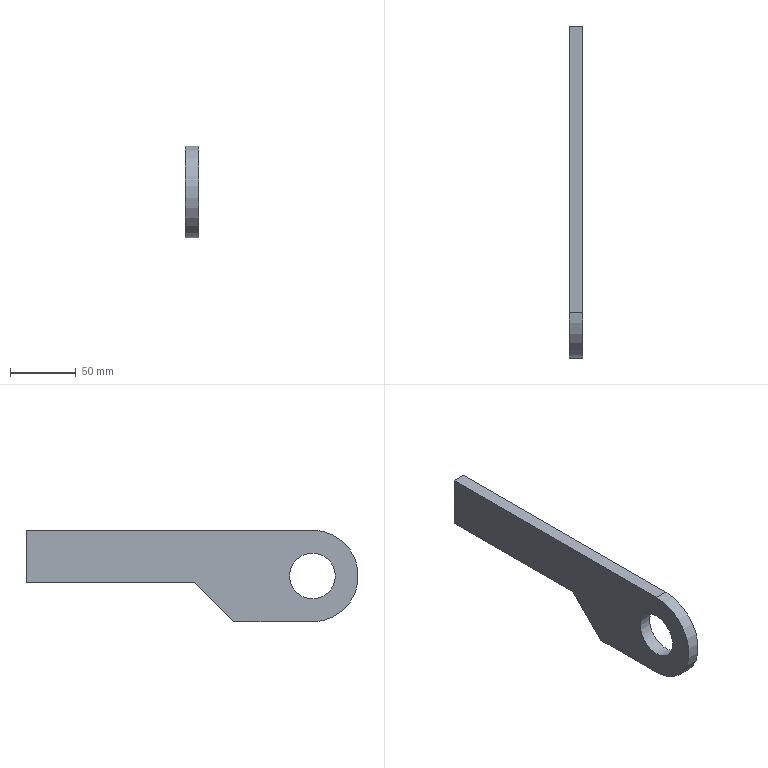Part | STEP file | body tilt cylinder mounting plate 1--000.001--20
240928 | 1 solid | 9 faces | box 10 x 253.506 x 70 mm | volume 119523 mm3 | plane 7 | cylinder 2 | commonest cylinder face diameters 35 x1 70 x1
STEP:
#1=CARTESIAN_POINT('',(0.,0.,0.));
#2=DIRECTION('',(0.,0.,1.));
#3=DIRECTION('',(1.,0.,0.));
#4=AXIS2_PLACEMENT_3D('',#1,#2,#3);
#5=CARTESIAN_POINT('',(-630.,216.,-35.));
#6=VERTEX_POINT('',#5);
#7=CARTESIAN_POINT('',(-630.,198.5,-35.));
#8=DIRECTION('',(1.,0.,0.));
#9=DIRECTION('',(0.,1.,0.));
#10=AXIS2_PLACEMENT_3D('',#7,#8,#9);
#11=CIRCLE('',#10,17.5);
#12=CARTESIAN_POINT('',(-630.,-284.,-150.));
#13=DIRECTION('',(1.,0.,0.));
#14=DIRECTION('',(0.,-1.,0.));
#15=AXIS2_PLACEMENT_3D('',#12,#13,#14);
#16=PLANE('',#15);
#17=CARTESIAN_POINT('',(-482.5,-115.));
#18=DIRECTION('',(-1.,0.));
#19=AXIS2_PLACEMENT_2D('',#17,#18);
#20=CIRCLE('',#19,17.5);
#21=(GEOMETRIC_REPRESENTATION_CONTEXT(2)PARAMETRIC_REPRESENTATION_CONTEXT()REPRESENTATION_CONTEXT('',''));
#22=DEFINITIONAL_REPRESENTATION('',(#20),#21);
#23=PCURVE('',#16,#22);
#24=CARTESIAN_POINT('',(-1050.,198.5,-35.));
#25=DIRECTION('',(1.,0.,0.));
#26=DIRECTION('',(0.,0.,1.));
#27=AXIS2_PLACEMENT_3D('',#24,#25,#26);
#28=CYLINDRICAL_SURFACE('',#27,17.5);
#29=CARTESIAN_POINT('',(4.712,420.));
#30=DIRECTION('',(1.,0.));
#31=VECTOR('',#30,1.);
#32=LINE('',#29,#31);
#33=(GEOMETRIC_REPRESENTATION_CONTEXT(2)PARAMETRIC_REPRESENTATION_CONTEXT()REPRESENTATION_CONTEXT('',''));
#34=DEFINITIONAL_REPRESENTATION('',(#32),#33);
#35=PCURVE('',#28,#34);
#36=SURFACE_CURVE('',#11,(#23,#35),.PCURVE_S1.);
#37=EDGE_CURVE('',#6,#6,#36,.T.);
#38=ORIENTED_EDGE('',*,*,#37,.F.);
#39=EDGE_LOOP('',(#38));
#40=FACE_BOUND('',#39,.T.);
#41=CARTESIAN_POINT('',(-630.,288.5,-40.));
#42=VERTEX_POINT('',#41);
#43=CARTESIAN_POINT('',(-630.,417.006,-40.));
#44=VERTEX_POINT('',#43);
#45=CARTESIAN_POINT('',(-630.,-284.,-40.));
#46=DIRECTION('',(0.,1.,0.));
#47=VECTOR('',#46,1.);
#48=LINE('',#45,#47);
#49=CARTESIAN_POINT('',(0.,-110.));
#50=DIRECTION('',(-1.,0.));
#51=VECTOR('',#50,1.);
#52=LINE('',#49,#51);
#53=(GEOMETRIC_REPRESENTATION_CONTEXT(2)PARAMETRIC_REPRESENTATION_CONTEXT()REPRESENTATION_CONTEXT('',''));
#54=DEFINITIONAL_REPRESENTATION('',(#52),#53);
#55=PCURVE('',#16,#54);
#56=CARTESIAN_POINT('',(-635.,288.5,-40.));
#57=DIRECTION('',(0.,0.,-1.));
#58=DIRECTION('',(1.,0.,0.));
#59=AXIS2_PLACEMENT_3D('',#56,#57,#58);
#60=PLANE('',#59);
#61=CARTESIAN_POINT('',(5.,572.5));
#62=DIRECTION('',(0.,-1.));
#63=VECTOR('',#62,1.);
#64=LINE('',#61,#63);
#65=(GEOMETRIC_REPRESENTATION_CONTEXT(2)PARAMETRIC_REPRESENTATION_CONTEXT()REPRESENTATION_CONTEXT('',''));
#66=DEFINITIONAL_REPRESENTATION('',(#64),#65);
#67=PCURVE('',#60,#66);
#68=SURFACE_CURVE('',#48,(#55,#67),.PCURVE_S1.);
#69=EDGE_CURVE('',#42,#44,#68,.T.);
#70=ORIENTED_EDGE('',*,*,#69,.T.);
#71=CARTESIAN_POINT('',(-630.,417.006,0.));
#72=VERTEX_POINT('',#71);
#73=CARTESIAN_POINT('',(-630.,417.006,-150.));
#74=DIRECTION('',(0.,0.,1.));
#75=VECTOR('',#74,1.);
#76=LINE('',#73,#75);
#77=CARTESIAN_POINT('',(-701.006,0.));
#78=DIRECTION('',(0.,-1.));
#79=VECTOR('',#78,1.);
#80=LINE('',#77,#79);
#81=(GEOMETRIC_REPRESENTATION_CONTEXT(2)PARAMETRIC_REPRESENTATION_CONTEXT()REPRESENTATION_CONTEXT('',''));
#82=DEFINITIONAL_REPRESENTATION('',(#80),#81);
#83=PCURVE('',#16,#82);
#84=CARTESIAN_POINT('',(-640.,417.006,0.));
#85=DIRECTION('',(0.,1.,0.));
#86=DIRECTION('',(0.,0.,-1.));
#87=AXIS2_PLACEMENT_3D('',#84,#85,#86);
#88=PLANE('',#87);
#89=CARTESIAN_POINT('',(150.,-10.));
#90=DIRECTION('',(-1.,0.));
#91=VECTOR('',#90,1.);
#92=LINE('',#89,#91);
#93=(GEOMETRIC_REPRESENTATION_CONTEXT(2)PARAMETRIC_REPRESENTATION_CONTEXT()REPRESENTATION_CONTEXT('',''));
#94=DEFINITIONAL_REPRESENTATION('',(#92),#93);
#95=PCURVE('',#88,#94);
#96=SURFACE_CURVE('',#76,(#83,#95),.PCURVE_S1.);
#97=EDGE_CURVE('',#44,#72,#96,.T.);
#98=ORIENTED_EDGE('',*,*,#97,.T.);
#99=CARTESIAN_POINT('',(-630.,198.5,0.));
#100=VERTEX_POINT('',#99);
#101=CARTESIAN_POINT('',(-630.,-488.,0.));
#102=DIRECTION('',(0.,1.,0.));
#103=VECTOR('',#102,1.);
#104=LINE('',#101,#103);
#105=CARTESIAN_POINT('',(204.,-150.));
#106=DIRECTION('',(-1.,0.));
#107=VECTOR('',#106,1.);
#108=LINE('',#105,#107);
#109=(GEOMETRIC_REPRESENTATION_CONTEXT(2)PARAMETRIC_REPRESENTATION_CONTEXT()REPRESENTATION_CONTEXT('',''));
#110=DEFINITIONAL_REPRESENTATION('',(#108),#109);
#111=PCURVE('',#16,#110);
#112=CARTESIAN_POINT('',(-750.,-488.,0.));
#113=DIRECTION('',(0.,0.,1.));
#114=DIRECTION('',(0.,1.,0.));
#115=AXIS2_PLACEMENT_3D('',#112,#113,#114);
#116=PLANE('',#115);
#117=CARTESIAN_POINT('',(0.,-120.));
#118=DIRECTION('',(1.,0.));
#119=VECTOR('',#118,1.);
#120=LINE('',#117,#119);
#121=(GEOMETRIC_REPRESENTATION_CONTEXT(2)PARAMETRIC_REPRESENTATION_CONTEXT()REPRESENTATION_CONTEXT('',''));
#122=DEFINITIONAL_REPRESENTATION('',(#120),#121);
#123=PCURVE('',#116,#122);
#124=SURFACE_CURVE('',#104,(#111,#123),.PCURVE_S1.);
#125=EDGE_CURVE('',#100,#72,#124,.T.);
#126=ORIENTED_EDGE('',*,*,#125,.F.);
#127=CARTESIAN_POINT('',(-630.,198.5,-70.));
#128=VERTEX_POINT('',#127);
#129=CARTESIAN_POINT('',(-630.,198.5,-35.));
#130=DIRECTION('',(1.,0.,0.));
#131=DIRECTION('',(0.,1.,0.));
#132=AXIS2_PLACEMENT_3D('',#129,#130,#131);
#133=CIRCLE('',#132,35.);
#134=CARTESIAN_POINT('',(-482.5,-115.));
#135=DIRECTION('',(-1.,0.));
#136=AXIS2_PLACEMENT_2D('',#134,#135);
#137=CIRCLE('',#136,35.);
#138=(GEOMETRIC_REPRESENTATION_CONTEXT(2)PARAMETRIC_REPRESENTATION_CONTEXT()REPRESENTATION_CONTEXT('',''));
#139=DEFINITIONAL_REPRESENTATION('',(#137),#138);
#140=PCURVE('',#16,#139);
#141=CARTESIAN_POINT('',(-700.,198.5,-35.));
#142=DIRECTION('',(-1.,0.,0.));
#143=DIRECTION('',(0.,0.,-1.));
#144=AXIS2_PLACEMENT_3D('',#141,#142,#143);
#145=CYLINDRICAL_SURFACE('',#144,35.);
#146=CARTESIAN_POINT('',(4.712,-70.));
#147=DIRECTION('',(-1.,0.));
#148=VECTOR('',#147,1.);
#149=LINE('',#146,#148);
#150=(GEOMETRIC_REPRESENTATION_CONTEXT(2)PARAMETRIC_REPRESENTATION_CONTEXT()REPRESENTATION_CONTEXT('',''));
#151=DEFINITIONAL_REPRESENTATION('',(#149),#150);
#152=PCURVE('',#145,#151);
#153=SURFACE_CURVE('',#133,(#140,#152),.PCURVE_S1.);
#154=EDGE_CURVE('',#100,#128,#153,.T.);
#155=ORIENTED_EDGE('',*,*,#154,.T.);
#156=CARTESIAN_POINT('',(-630.,258.5,-70.));
#157=VERTEX_POINT('',#156);
#158=CARTESIAN_POINT('',(-630.,198.5,-70.));
#159=DIRECTION('',(0.,-1.,0.));
#160=VECTOR('',#159,1.);
#161=LINE('',#158,#160);
#162=CARTESIAN_POINT('',(-482.5,-80.));
#163=DIRECTION('',(1.,0.));
#164=VECTOR('',#163,1.);
#165=LINE('',#162,#164);
#166=(GEOMETRIC_REPRESENTATION_CONTEXT(2)PARAMETRIC_REPRESENTATION_CONTEXT()REPRESENTATION_CONTEXT('',''));
#167=DEFINITIONAL_REPRESENTATION('',(#165),#166);
#168=PCURVE('',#16,#167);
#169=CARTESIAN_POINT('',(-700.,198.5,-70.));
#170=DIRECTION('',(0.,0.,-1.));
#171=DIRECTION('',(1.,0.,0.));
#172=AXIS2_PLACEMENT_3D('',#169,#170,#171);
#173=PLANE('',#172);
#174=CARTESIAN_POINT('',(70.,0.));
#175=DIRECTION('',(0.,1.));
#176=VECTOR('',#175,1.);
#177=LINE('',#174,#176);
#178=(GEOMETRIC_REPRESENTATION_CONTEXT(2)PARAMETRIC_REPRESENTATION_CONTEXT()REPRESENTATION_CONTEXT('',''));
#179=DEFINITIONAL_REPRESENTATION('',(#177),#178);
#180=PCURVE('',#173,#179);
#181=SURFACE_CURVE('',#161,(#168,#180),.PCURVE_S1.);
#182=EDGE_CURVE('',#157,#128,#181,.T.);
#183=ORIENTED_EDGE('',*,*,#182,.F.);
#184=CARTESIAN_POINT('',(-630.,-102.75,-431.25));
#185=DIRECTION('',(0.,0.7071,0.7071));
#186=VECTOR('',#185,1.);
#187=LINE('',#184,#186);
#188=CARTESIAN_POINT('',(-181.25,281.25));
#189=DIRECTION('',(-0.7071,-0.7071));
#190=VECTOR('',#189,1.);
#191=LINE('',#188,#190);
#192=(GEOMETRIC_REPRESENTATION_CONTEXT(2)PARAMETRIC_REPRESENTATION_CONTEXT()REPRESENTATION_CONTEXT('',''));
#193=DEFINITIONAL_REPRESENTATION('',(#191),#192);
#194=PCURVE('',#16,#193);
#195=CARTESIAN_POINT('',(600.173,268.5,-60.));
#196=DIRECTION('',(0.,-0.7071,0.7071));
#197=DIRECTION('',(1.,0.,0.));
#198=AXIS2_PLACEMENT_3D('',#195,#196,#197);
#199=PLANE('',#198);
#200=CARTESIAN_POINT('',(-1230.173,-525.027));
#201=DIRECTION('',(0.,1.));
#202=VECTOR('',#201,1.);
#203=LINE('',#200,#202);
#204=(GEOMETRIC_REPRESENTATION_CONTEXT(2)PARAMETRIC_REPRESENTATION_CONTEXT()REPRESENTATION_CONTEXT('',''));
#205=DEFINITIONAL_REPRESENTATION('',(#203),#204);
#206=PCURVE('',#199,#205);
#207=SURFACE_CURVE('',#187,(#194,#206),.PCURVE_S1.);
#208=EDGE_CURVE('',#157,#42,#207,.T.);
#209=ORIENTED_EDGE('',*,*,#208,.T.);
#210=EDGE_LOOP('',(#70,#98,#126,#155,#183,#209));
#211=FACE_BOUND('',#210,.T.);
#212=ADVANCED_FACE('',(#40,#211),#16,.T.);
#213=ORIENTED_EDGE('',*,*,#125,.T.);
#214=CARTESIAN_POINT('',(-640.,417.006,0.));
#215=VERTEX_POINT('',#214);
#216=CARTESIAN_POINT('',(-750.,417.006,0.));
#217=DIRECTION('',(-1.,0.,0.));
#218=VECTOR('',#217,1.);
#219=LINE('',#216,#218);
#220=CARTESIAN_POINT('',(905.006,0.));
#221=DIRECTION('',(0.,1.));
#222=VECTOR('',#221,1.);
#223=LINE('',#220,#222);
#224=(GEOMETRIC_REPRESENTATION_CONTEXT(2)PARAMETRIC_REPRESENTATION_CONTEXT()REPRESENTATION_CONTEXT('',''));
#225=DEFINITIONAL_REPRESENTATION('',(#223),#224);
#226=PCURVE('',#116,#225);
#227=CARTESIAN_POINT('',(0.,110.));
#228=DIRECTION('',(0.,1.));
#229=VECTOR('',#228,1.);
#230=LINE('',#227,#229);
#231=(GEOMETRIC_REPRESENTATION_CONTEXT(2)PARAMETRIC_REPRESENTATION_CONTEXT()REPRESENTATION_CONTEXT('',''));
#232=DEFINITIONAL_REPRESENTATION('',(#230),#231);
#233=PCURVE('',#88,#232);
#234=SURFACE_CURVE('',#219,(#226,#233),.PCURVE_S1.);
#235=EDGE_CURVE('',#72,#215,#234,.T.);
#236=ORIENTED_EDGE('',*,*,#235,.T.);
#237=CARTESIAN_POINT('',(-640.,198.5,0.));
#238=VERTEX_POINT('',#237);
#239=CARTESIAN_POINT('',(-640.,-488.,0.));
#240=DIRECTION('',(0.,-1.,0.));
#241=VECTOR('',#240,1.);
#242=LINE('',#239,#241);
#243=CARTESIAN_POINT('',(0.,-110.));
#244=DIRECTION('',(-1.,0.));
#245=VECTOR('',#244,1.);
#246=LINE('',#243,#245);
#247=(GEOMETRIC_REPRESENTATION_CONTEXT(2)PARAMETRIC_REPRESENTATION_CONTEXT()REPRESENTATION_CONTEXT('',''));
#248=DEFINITIONAL_REPRESENTATION('',(#246),#247);
#249=PCURVE('',#116,#248);
#250=CARTESIAN_POINT('',(-640.,-284.,-150.));
#251=DIRECTION('',(-1.,0.,0.));
#252=DIRECTION('',(0.,1.,0.));
#253=AXIS2_PLACEMENT_3D('',#250,#251,#252);
#254=PLANE('',#253);
#255=CARTESIAN_POINT('',(-204.,-150.));
#256=DIRECTION('',(-1.,0.));
#257=VECTOR('',#256,1.);
#258=LINE('',#255,#257);
#259=(GEOMETRIC_REPRESENTATION_CONTEXT(2)PARAMETRIC_REPRESENTATION_CONTEXT()REPRESENTATION_CONTEXT('',''));
#260=DEFINITIONAL_REPRESENTATION('',(#258),#259);
#261=PCURVE('',#254,#260);
#262=SURFACE_CURVE('',#242,(#249,#261),.PCURVE_S1.);
#263=EDGE_CURVE('',#215,#238,#262,.T.);
#264=ORIENTED_EDGE('',*,*,#263,.T.);
#265=CARTESIAN_POINT('',(-750.,198.5,0.));
#266=DIRECTION('',(1.,0.,0.));
#267=VECTOR('',#266,1.);
#268=LINE('',#265,#267);
#269=CARTESIAN_POINT('',(686.5,0.));
#270=DIRECTION('',(0.,-1.));
#271=VECTOR('',#270,1.);
#272=LINE('',#269,#271);
#273=(GEOMETRIC_REPRESENTATION_CONTEXT(2)PARAMETRIC_REPRESENTATION_CONTEXT()REPRESENTATION_CONTEXT('',''));
#274=DEFINITIONAL_REPRESENTATION('',(#272),#273);
#275=PCURVE('',#116,#274);
#276=CARTESIAN_POINT('',(3.142,50.));
#277=DIRECTION('',(0.,-1.));
#278=VECTOR('',#277,1.);
#279=LINE('',#276,#278);
#280=(GEOMETRIC_REPRESENTATION_CONTEXT(2)PARAMETRIC_REPRESENTATION_CONTEXT()REPRESENTATION_CONTEXT('',''));
#281=DEFINITIONAL_REPRESENTATION('',(#279),#280);
#282=PCURVE('',#145,#281);
#283=SURFACE_CURVE('',#268,(#275,#282),.PCURVE_S1.);
#284=EDGE_CURVE('',#238,#100,#283,.T.);
#285=ORIENTED_EDGE('',*,*,#284,.T.);
#286=EDGE_LOOP('',(#213,#236,#264,#285));
#287=FACE_BOUND('',#286,.T.);
#288=ADVANCED_FACE('',(#287),#116,.T.);
#289=CARTESIAN_POINT('',(-640.,417.006,-40.));
#290=VERTEX_POINT('',#289);
#291=CARTESIAN_POINT('',(-640.,288.5,-40.));
#292=VERTEX_POINT('',#291);
#293=CARTESIAN_POINT('',(-640.,-284.,-40.));
#294=DIRECTION('',(0.,-1.,0.));
#295=VECTOR('',#294,1.);
#296=LINE('',#293,#295);
#297=CARTESIAN_POINT('',(-5.,572.5));
#298=DIRECTION('',(0.,1.));
#299=VECTOR('',#298,1.);
#300=LINE('',#297,#299);
#301=(GEOMETRIC_REPRESENTATION_CONTEXT(2)PARAMETRIC_REPRESENTATION_CONTEXT()REPRESENTATION_CONTEXT('',''));
#302=DEFINITIONAL_REPRESENTATION('',(#300),#301);
#303=PCURVE('',#60,#302);
#304=CARTESIAN_POINT('',(0.,-110.));
#305=DIRECTION('',(-1.,0.));
#306=VECTOR('',#305,1.);
#307=LINE('',#304,#306);
#308=(GEOMETRIC_REPRESENTATION_CONTEXT(2)PARAMETRIC_REPRESENTATION_CONTEXT()REPRESENTATION_CONTEXT('',''));
#309=DEFINITIONAL_REPRESENTATION('',(#307),#308);
#310=PCURVE('',#254,#309);
#311=SURFACE_CURVE('',#296,(#303,#310),.PCURVE_S1.);
#312=EDGE_CURVE('',#290,#292,#311,.T.);
#313=ORIENTED_EDGE('',*,*,#312,.F.);
#314=CARTESIAN_POINT('',(-635.,417.006,-40.));
#315=DIRECTION('',(1.,0.,0.));
#316=VECTOR('',#315,1.);
#317=LINE('',#314,#316);
#318=CARTESIAN_POINT('',(0.,-128.506));
#319=DIRECTION('',(1.,0.));
#320=VECTOR('',#319,1.);
#321=LINE('',#318,#320);
#322=(GEOMETRIC_REPRESENTATION_CONTEXT(2)PARAMETRIC_REPRESENTATION_CONTEXT()REPRESENTATION_CONTEXT('',''));
#323=DEFINITIONAL_REPRESENTATION('',(#321),#322);
#324=PCURVE('',#60,#323);
#325=CARTESIAN_POINT('',(40.,-5.));
#326=DIRECTION('',(0.,-1.));
#327=VECTOR('',#326,1.);
#328=LINE('',#325,#327);
#329=(GEOMETRIC_REPRESENTATION_CONTEXT(2)PARAMETRIC_REPRESENTATION_CONTEXT()REPRESENTATION_CONTEXT('',''));
#330=DEFINITIONAL_REPRESENTATION('',(#328),#329);
#331=PCURVE('',#88,#330);
#332=SURFACE_CURVE('',#317,(#324,#331),.PCURVE_S1.);
#333=EDGE_CURVE('',#290,#44,#332,.T.);
#334=ORIENTED_EDGE('',*,*,#333,.T.);
#335=ORIENTED_EDGE('',*,*,#69,.F.);
#336=CARTESIAN_POINT('',(-635.,288.5,-40.));
#337=DIRECTION('',(1.,0.,0.));
#338=VECTOR('',#337,1.);
#339=LINE('',#336,#338);
#340=CARTESIAN_POINT('',(0.,0.));
#341=DIRECTION('',(1.,0.));
#342=VECTOR('',#341,1.);
#343=LINE('',#340,#342);
#344=(GEOMETRIC_REPRESENTATION_CONTEXT(2)PARAMETRIC_REPRESENTATION_CONTEXT()REPRESENTATION_CONTEXT('',''));
#345=DEFINITIONAL_REPRESENTATION('',(#343),#344);
#346=PCURVE('',#60,#345);
#347=CARTESIAN_POINT('',(-1235.173,28.284));
#348=DIRECTION('',(1.,0.));
#349=VECTOR('',#348,1.);
#350=LINE('',#347,#349);
#351=(GEOMETRIC_REPRESENTATION_CONTEXT(2)PARAMETRIC_REPRESENTATION_CONTEXT()REPRESENTATION_CONTEXT('',''));
#352=DEFINITIONAL_REPRESENTATION('',(#350),#351);
#353=PCURVE('',#199,#352);
#354=SURFACE_CURVE('',#339,(#346,#353),.PCURVE_S1.);
#355=EDGE_CURVE('',#292,#42,#354,.T.);
#356=ORIENTED_EDGE('',*,*,#355,.F.);
#357=EDGE_LOOP('',(#313,#334,#335,#356));
#358=FACE_BOUND('',#357,.T.);
#359=ADVANCED_FACE('',(#358),#60,.T.);
#360=CARTESIAN_POINT('',(-640.,181.,-35.));
#361=VERTEX_POINT('',#360);
#362=CARTESIAN_POINT('',(-640.,216.,-35.));
#363=VERTEX_POINT('',#362);
#364=CARTESIAN_POINT('',(-640.,198.5,-35.));
#365=DIRECTION('',(-1.,0.,0.));
#366=DIRECTION('',(0.,-1.,0.));
#367=AXIS2_PLACEMENT_3D('',#364,#365,#366);
#368=CIRCLE('',#367,17.5);
#369=CARTESIAN_POINT('',(482.5,-115.));
#370=DIRECTION('',(-1.,0.));
#371=AXIS2_PLACEMENT_2D('',#369,#370);
#372=CIRCLE('',#371,17.5);
#373=(GEOMETRIC_REPRESENTATION_CONTEXT(2)PARAMETRIC_REPRESENTATION_CONTEXT()REPRESENTATION_CONTEXT('',''));
#374=DEFINITIONAL_REPRESENTATION('',(#372),#373);
#375=PCURVE('',#254,#374);
#376=CARTESIAN_POINT('',(7.854,410.));
#377=DIRECTION('',(-1.,0.));
#378=VECTOR('',#377,1.);
#379=LINE('',#376,#378);
#380=(GEOMETRIC_REPRESENTATION_CONTEXT(2)PARAMETRIC_REPRESENTATION_CONTEXT()REPRESENTATION_CONTEXT('',''));
#381=DEFINITIONAL_REPRESENTATION('',(#379),#380);
#382=PCURVE('',#28,#381);
#383=SURFACE_CURVE('',#368,(#375,#382),.PCURVE_S1.);
#384=EDGE_CURVE('',#361,#363,#383,.T.);
#385=ORIENTED_EDGE('',*,*,#384,.F.);
#386=CARTESIAN_POINT('',(-640.,198.5,-35.));
#387=DIRECTION('',(-1.,0.,0.));
#388=DIRECTION('',(0.,-1.,0.));
#389=AXIS2_PLACEMENT_3D('',#386,#387,#388);
#390=CIRCLE('',#389,17.5);
#391=CARTESIAN_POINT('',(482.5,-115.));
#392=DIRECTION('',(-1.,0.));
#393=AXIS2_PLACEMENT_2D('',#391,#392);
#394=CIRCLE('',#393,17.5);
#395=(GEOMETRIC_REPRESENTATION_CONTEXT(2)PARAMETRIC_REPRESENTATION_CONTEXT()REPRESENTATION_CONTEXT('',''));
#396=DEFINITIONAL_REPRESENTATION('',(#394),#395);
#397=PCURVE('',#254,#396);
#398=CARTESIAN_POINT('',(14.137,410.));
#399=DIRECTION('',(-1.,0.));
#400=VECTOR('',#399,1.);
#401=LINE('',#398,#400);
#402=(GEOMETRIC_REPRESENTATION_CONTEXT(2)PARAMETRIC_REPRESENTATION_CONTEXT()REPRESENTATION_CONTEXT('',''));
#403=DEFINITIONAL_REPRESENTATION('',(#401),#402);
#404=PCURVE('',#28,#403);
#405=SURFACE_CURVE('',#390,(#397,#404),.PCURVE_S1.);
#406=EDGE_CURVE('',#363,#361,#405,.T.);
#407=ORIENTED_EDGE('',*,*,#406,.F.);
#408=EDGE_LOOP('',(#385,#407));
#409=FACE_BOUND('',#408,.T.);
#410=CARTESIAN_POINT('',(-640.,417.006,0.000000001));
#411=DIRECTION('',(0.,0.,1.));
#412=VECTOR('',#411,1.);
#413=LINE('',#410,#412);
#414=CARTESIAN_POINT('',(701.006,-150.));
#415=DIRECTION('',(0.,-1.));
#416=VECTOR('',#415,1.);
#417=LINE('',#414,#416);
#418=(GEOMETRIC_REPRESENTATION_CONTEXT(2)PARAMETRIC_REPRESENTATION_CONTEXT()REPRESENTATION_CONTEXT('',''));
#419=DEFINITIONAL_REPRESENTATION('',(#417),#418);
#420=PCURVE('',#254,#419);
#421=CARTESIAN_POINT('',(-0.000000001,0.));
#422=DIRECTION('',(-1.,0.));
#423=VECTOR('',#422,1.);
#424=LINE('',#421,#423);
#425=(GEOMETRIC_REPRESENTATION_CONTEXT(2)PARAMETRIC_REPRESENTATION_CONTEXT()REPRESENTATION_CONTEXT('',''));
#426=DEFINITIONAL_REPRESENTATION('',(#424),#425);
#427=PCURVE('',#88,#426);
#428=SURFACE_CURVE('',#413,(#420,#427),.PCURVE_S1.);
#429=EDGE_CURVE('',#290,#215,#428,.T.);
#430=ORIENTED_EDGE('',*,*,#429,.F.);
#431=ORIENTED_EDGE('',*,*,#312,.T.);
#432=CARTESIAN_POINT('',(-640.,258.5,-70.));
#433=VERTEX_POINT('',#432);
#434=CARTESIAN_POINT('',(-640.,-102.75,-431.25));
#435=DIRECTION('',(0.,-0.7071,-0.7071));
#436=VECTOR('',#435,1.);
#437=LINE('',#434,#436);
#438=CARTESIAN_POINT('',(181.25,281.25));
#439=DIRECTION('',(-0.7071,0.7071));
#440=VECTOR('',#439,1.);
#441=LINE('',#438,#440);
#442=(GEOMETRIC_REPRESENTATION_CONTEXT(2)PARAMETRIC_REPRESENTATION_CONTEXT()REPRESENTATION_CONTEXT('',''));
#443=DEFINITIONAL_REPRESENTATION('',(#441),#442);
#444=PCURVE('',#254,#443);
#445=CARTESIAN_POINT('',(-1240.173,-525.027));
#446=DIRECTION('',(0.,-1.));
#447=VECTOR('',#446,1.);
#448=LINE('',#445,#447);
#449=(GEOMETRIC_REPRESENTATION_CONTEXT(2)PARAMETRIC_REPRESENTATION_CONTEXT()REPRESENTATION_CONTEXT('',''));
#450=DEFINITIONAL_REPRESENTATION('',(#448),#449);
#451=PCURVE('',#199,#450);
#452=SURFACE_CURVE('',#437,(#444,#451),.PCURVE_S1.);
#453=EDGE_CURVE('',#292,#433,#452,.T.);
#454=ORIENTED_EDGE('',*,*,#453,.T.);
#455=CARTESIAN_POINT('',(-640.,198.5,-70.));
#456=VERTEX_POINT('',#455);
#457=CARTESIAN_POINT('',(-640.,198.5,-70.));
#458=DIRECTION('',(0.,1.,0.));
#459=VECTOR('',#458,1.);
#460=LINE('',#457,#459);
#461=CARTESIAN_POINT('',(482.5,-80.));
#462=DIRECTION('',(1.,0.));
#463=VECTOR('',#462,1.);
#464=LINE('',#461,#463);
#465=(GEOMETRIC_REPRESENTATION_CONTEXT(2)PARAMETRIC_REPRESENTATION_CONTEXT()REPRESENTATION_CONTEXT('',''));
#466=DEFINITIONAL_REPRESENTATION('',(#464),#465);
#467=PCURVE('',#254,#466);
#468=CARTESIAN_POINT('',(60.,0.));
#469=DIRECTION('',(0.,-1.));
#470=VECTOR('',#469,1.);
#471=LINE('',#468,#470);
#472=(GEOMETRIC_REPRESENTATION_CONTEXT(2)PARAMETRIC_REPRESENTATION_CONTEXT()REPRESENTATION_CONTEXT('',''));
#473=DEFINITIONAL_REPRESENTATION('',(#471),#472);
#474=PCURVE('',#173,#473);
#475=SURFACE_CURVE('',#460,(#467,#474),.PCURVE_S1.);
#476=EDGE_CURVE('',#456,#433,#475,.T.);
#477=ORIENTED_EDGE('',*,*,#476,.F.);
#478=CARTESIAN_POINT('',(-640.,198.5,-35.));
#479=DIRECTION('',(-1.,0.,0.));
#480=DIRECTION('',(0.,-1.,0.));
#481=AXIS2_PLACEMENT_3D('',#478,#479,#480);
#482=CIRCLE('',#481,35.);
#483=CARTESIAN_POINT('',(482.5,-115.));
#484=DIRECTION('',(-1.,0.));
#485=AXIS2_PLACEMENT_2D('',#483,#484);
#486=CIRCLE('',#485,35.);
#487=(GEOMETRIC_REPRESENTATION_CONTEXT(2)PARAMETRIC_REPRESENTATION_CONTEXT()REPRESENTATION_CONTEXT('',''));
#488=DEFINITIONAL_REPRESENTATION('',(#486),#487);
#489=PCURVE('',#254,#488);
#490=CARTESIAN_POINT('',(-4.712,-60.));
#491=DIRECTION('',(1.,0.));
#492=VECTOR('',#491,1.);
#493=LINE('',#490,#492);
#494=(GEOMETRIC_REPRESENTATION_CONTEXT(2)PARAMETRIC_REPRESENTATION_CONTEXT()REPRESENTATION_CONTEXT('',''));
#495=DEFINITIONAL_REPRESENTATION('',(#493),#494);
#496=PCURVE('',#145,#495);
#497=SURFACE_CURVE('',#482,(#489,#496),.PCURVE_S1.);
#498=EDGE_CURVE('',#456,#238,#497,.T.);
#499=ORIENTED_EDGE('',*,*,#498,.T.);
#500=ORIENTED_EDGE('',*,*,#263,.F.);
#501=EDGE_LOOP('',(#430,#431,#454,#477,#499,#500));
#502=FACE_BOUND('',#501,.T.);
#503=ADVANCED_FACE('',(#409,#502),#254,.T.);
#504=ORIENTED_EDGE('',*,*,#498,.F.);
#505=CARTESIAN_POINT('',(-700.,198.5,-70.));
#506=DIRECTION('',(-1.,0.,0.));
#507=VECTOR('',#506,1.);
#508=LINE('',#505,#507);
#509=CARTESIAN_POINT('',(0.,0.));
#510=DIRECTION('',(0.,1.));
#511=VECTOR('',#510,1.);
#512=LINE('',#509,#511);
#513=(GEOMETRIC_REPRESENTATION_CONTEXT(2)PARAMETRIC_REPRESENTATION_CONTEXT()REPRESENTATION_CONTEXT('',''));
#514=DEFINITIONAL_REPRESENTATION('',(#512),#513);
#515=PCURVE('',#145,#514);
#516=CARTESIAN_POINT('',(0.,0.));
#517=DIRECTION('',(-1.,0.));
#518=VECTOR('',#517,1.);
#519=LINE('',#516,#518);
#520=(GEOMETRIC_REPRESENTATION_CONTEXT(2)PARAMETRIC_REPRESENTATION_CONTEXT()REPRESENTATION_CONTEXT('',''));
#521=DEFINITIONAL_REPRESENTATION('',(#519),#520);
#522=PCURVE('',#173,#521);
#523=SURFACE_CURVE('',#508,(#515,#522),.PCURVE_S1.);
#524=EDGE_CURVE('',#128,#456,#523,.T.);
#525=ORIENTED_EDGE('',*,*,#524,.F.);
#526=ORIENTED_EDGE('',*,*,#154,.F.);
#527=ORIENTED_EDGE('',*,*,#284,.F.);
#528=EDGE_LOOP('',(#504,#525,#526,#527));
#529=FACE_BOUND('',#528,.T.);
#530=ADVANCED_FACE('',(#529),#145,.T.);
#531=ORIENTED_EDGE('',*,*,#406,.F.);
#532=CARTESIAN_POINT('',(-640.,216.,-35.));
#533=CARTESIAN_POINT('',(-630.,216.,-35.));
#534=B_SPLINE_CURVE_WITH_KNOTS('',1,(#532,#533),.UNSPECIFIED.,.F.,.F.,(2,2),(410.,420.),.PIECEWISE_BEZIER_KNOTS.);
#535=CARTESIAN_POINT('',(10.996,0.));
#536=DIRECTION('',(0.,1.));
#537=VECTOR('',#536,1.);
#538=LINE('',#535,#537);
#539=(GEOMETRIC_REPRESENTATION_CONTEXT(2)PARAMETRIC_REPRESENTATION_CONTEXT()REPRESENTATION_CONTEXT('',''));
#540=DEFINITIONAL_REPRESENTATION('',(#538),#539);
#541=PCURVE('',#28,#540);
#542=CARTESIAN_POINT('',(4.712,0.));
#543=DIRECTION('',(0.,1.));
#544=VECTOR('',#543,1.);
#545=LINE('',#542,#544);
#546=(GEOMETRIC_REPRESENTATION_CONTEXT(2)PARAMETRIC_REPRESENTATION_CONTEXT()REPRESENTATION_CONTEXT('',''));
#547=DEFINITIONAL_REPRESENTATION('',(#545),#546);
#548=PCURVE('',#28,#547);
#549=SEAM_CURVE('',#534,(#541,#548),.PCURVE_S1.);
#550=EDGE_CURVE('',#363,#6,#549,.T.);
#551=ORIENTED_EDGE('',*,*,#550,.T.);
#552=ORIENTED_EDGE('',*,*,#37,.F.);
#553=ORIENTED_EDGE('',*,*,#550,.F.);
#554=ORIENTED_EDGE('',*,*,#384,.F.);
#555=EDGE_LOOP('',(#531,#551,#552,#553,#554));
#556=FACE_BOUND('',#555,.F.);
#557=ADVANCED_FACE('',(#556),#28,.F.);
#558=ORIENTED_EDGE('',*,*,#476,.T.);
#559=CARTESIAN_POINT('',(-700.,258.5,-70.));
#560=DIRECTION('',(1.,0.,0.));
#561=VECTOR('',#560,1.);
#562=LINE('',#559,#561);
#563=CARTESIAN_POINT('',(0.,-60.));
#564=DIRECTION('',(1.,0.));
#565=VECTOR('',#564,1.);
#566=LINE('',#563,#565);
#567=(GEOMETRIC_REPRESENTATION_CONTEXT(2)PARAMETRIC_REPRESENTATION_CONTEXT()REPRESENTATION_CONTEXT('',''));
#568=DEFINITIONAL_REPRESENTATION('',(#566),#567);
#569=PCURVE('',#173,#568);
#570=CARTESIAN_POINT('',(-1300.173,-14.142));
#571=DIRECTION('',(1.,0.));
#572=VECTOR('',#571,1.);
#573=LINE('',#570,#572);
#574=(GEOMETRIC_REPRESENTATION_CONTEXT(2)PARAMETRIC_REPRESENTATION_CONTEXT()REPRESENTATION_CONTEXT('',''));
#575=DEFINITIONAL_REPRESENTATION('',(#573),#574);
#576=PCURVE('',#199,#575);
#577=SURFACE_CURVE('',#562,(#569,#576),.PCURVE_S1.);
#578=EDGE_CURVE('',#433,#157,#577,.T.);
#579=ORIENTED_EDGE('',*,*,#578,.T.);
#580=ORIENTED_EDGE('',*,*,#182,.T.);
#581=ORIENTED_EDGE('',*,*,#524,.T.);
#582=EDGE_LOOP('',(#558,#579,#580,#581));
#583=FACE_BOUND('',#582,.T.);
#584=ADVANCED_FACE('',(#583),#173,.T.);
#585=ORIENTED_EDGE('',*,*,#208,.F.);
#586=ORIENTED_EDGE('',*,*,#578,.F.);
#587=ORIENTED_EDGE('',*,*,#453,.F.);
#588=ORIENTED_EDGE('',*,*,#355,.T.);
#589=EDGE_LOOP('',(#585,#586,#587,#588));
#590=FACE_BOUND('',#589,.T.);
#591=ADVANCED_FACE('',(#590),#199,.F.);
#592=ORIENTED_EDGE('',*,*,#97,.F.);
#593=ORIENTED_EDGE('',*,*,#333,.F.);
#594=ORIENTED_EDGE('',*,*,#429,.T.);
#595=ORIENTED_EDGE('',*,*,#235,.F.);
#596=EDGE_LOOP('',(#592,#593,#594,#595));
#597=FACE_BOUND('',#596,.T.);
#598=ADVANCED_FACE('',(#597),#88,.T.);
#599=CLOSED_SHELL('',(#212,#288,#359,#503,#530,#557,#584,#591,#598));
#600=MANIFOLD_SOLID_BREP('',#599);
#601=(LENGTH_UNIT()NAMED_UNIT(*)SI_UNIT(.MILLI.,.METRE.));
#602=UNCERTAINTY_MEASURE_WITH_UNIT(LENGTH_MEASURE(0.000001),#601,'','');
#603=(NAMED_UNIT(*)PLANE_ANGLE_UNIT()SI_UNIT($,.RADIAN.));
#604=(NAMED_UNIT(*)SI_UNIT($,.STERADIAN.)SOLID_ANGLE_UNIT());
#605=(GEOMETRIC_REPRESENTATION_CONTEXT(3)GLOBAL_UNCERTAINTY_ASSIGNED_CONTEXT((#602))GLOBAL_UNIT_ASSIGNED_CONTEXT((#601,#603,#604))REPRESENTATION_CONTEXT('',''));
#606=ADVANCED_BREP_SHAPE_REPRESENTATION('',(#4,#600),#605);